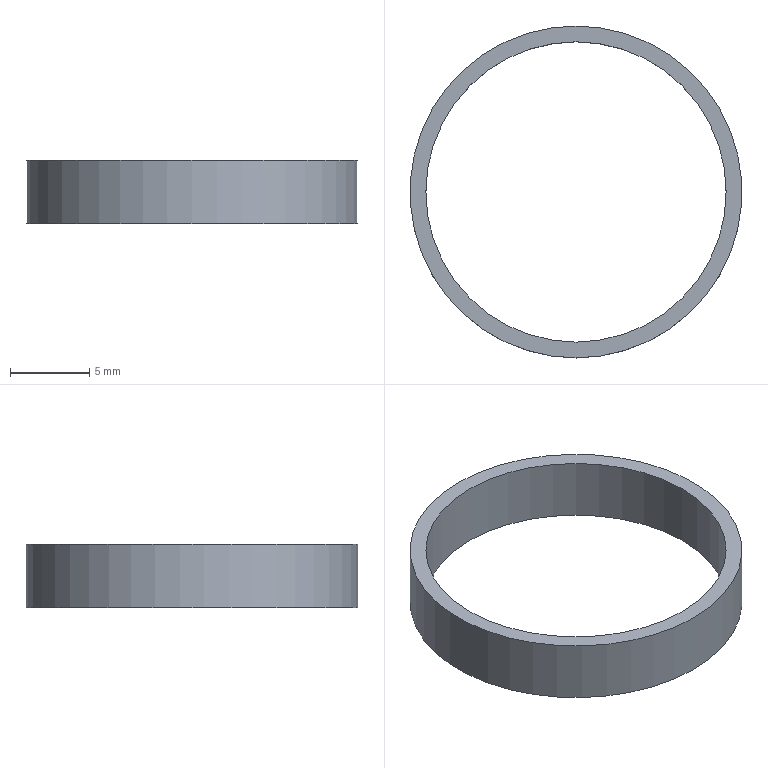Part | NX | features solid 2 | 1 solid | 4 faces | box 21 x 21 x 4 mm | volume 251.327 mm3 | cylinder 2 | plane 2 | commonest cylinder face diameters 19 x1 21 x1
STEP:
#1=CARTESIAN_POINT('',(254.748,69.5,-15.));
#2=VERTEX_POINT('',#1);
#3=CARTESIAN_POINT('',(254.748,60.,-15.));
#4=DIRECTION('',(0.,0.,-1.));
#5=DIRECTION('',(0.,1.,0.));
#6=AXIS2_PLACEMENT_3D('',#3,#4,#5);
#7=CIRCLE('',#6,9.5);
#8=EDGE_CURVE('',#2,#2,#7,.T.);
#9=ORIENTED_EDGE('',*,*,#8,.T.);
#10=EDGE_LOOP('',(#9));
#11=FACE_BOUND('',#10,.T.);
#12=CARTESIAN_POINT('',(254.748,69.5,-11.));
#13=VERTEX_POINT('',#12);
#14=CARTESIAN_POINT('',(254.748,60.,-11.));
#15=DIRECTION('',(0.,0.,-1.));
#16=DIRECTION('',(0.,1.,0.));
#17=AXIS2_PLACEMENT_3D('',#14,#15,#16);
#18=CIRCLE('',#17,9.5);
#19=EDGE_CURVE('',#13,#13,#18,.T.);
#20=ORIENTED_EDGE('',*,*,#19,.F.);
#21=EDGE_LOOP('',(#20));
#22=FACE_BOUND('',#21,.T.);
#23=CARTESIAN_POINT('',(254.748,60.,-15.));
#24=DIRECTION('',(0.,0.,1.));
#25=DIRECTION('',(0.,1.,0.));
#26=AXIS2_PLACEMENT_3D('',#23,#24,#25);
#27=CYLINDRICAL_SURFACE('',#26,9.5);
#28=ADVANCED_FACE('',(#11,#22),#27,.F.);
#29=CARTESIAN_POINT('',(254.748,70.5,-15.));
#30=VERTEX_POINT('',#29);
#31=CARTESIAN_POINT('',(254.748,60.,-15.));
#32=DIRECTION('',(0.,0.,-1.));
#33=DIRECTION('',(0.,1.,0.));
#34=AXIS2_PLACEMENT_3D('',#31,#32,#33);
#35=CIRCLE('',#34,10.5);
#36=EDGE_CURVE('',#30,#30,#35,.T.);
#37=ORIENTED_EDGE('',*,*,#36,.F.);
#38=EDGE_LOOP('',(#37));
#39=FACE_BOUND('',#38,.T.);
#40=CARTESIAN_POINT('',(254.748,70.5,-11.));
#41=VERTEX_POINT('',#40);
#42=CARTESIAN_POINT('',(254.748,60.,-11.));
#43=DIRECTION('',(0.,0.,-1.));
#44=DIRECTION('',(0.,1.,0.));
#45=AXIS2_PLACEMENT_3D('',#42,#43,#44);
#46=CIRCLE('',#45,10.5);
#47=EDGE_CURVE('',#41,#41,#46,.T.);
#48=ORIENTED_EDGE('',*,*,#47,.T.);
#49=EDGE_LOOP('',(#48));
#50=FACE_BOUND('',#49,.T.);
#51=CARTESIAN_POINT('',(254.748,60.,-15.));
#52=DIRECTION('',(0.,0.,1.));
#53=DIRECTION('',(0.,1.,0.));
#54=AXIS2_PLACEMENT_3D('',#51,#52,#53);
#55=CYLINDRICAL_SURFACE('',#54,10.5);
#56=ADVANCED_FACE('',(#39,#50),#55,.T.);
#57=ORIENTED_EDGE('',*,*,#8,.F.);
#58=EDGE_LOOP('',(#57));
#59=FACE_BOUND('',#58,.T.);
#60=ORIENTED_EDGE('',*,*,#36,.T.);
#61=EDGE_LOOP('',(#60));
#62=FACE_BOUND('',#61,.T.);
#63=CARTESIAN_POINT('',(254.748,60.,-15.));
#64=DIRECTION('',(0.,0.,-1.));
#65=DIRECTION('',(0.,-1.,0.));
#66=AXIS2_PLACEMENT_3D('',#63,#64,#65);
#67=PLANE('',#66);
#68=ADVANCED_FACE('',(#59,#62),#67,.T.);
#69=ORIENTED_EDGE('',*,*,#19,.T.);
#70=EDGE_LOOP('',(#69));
#71=FACE_BOUND('',#70,.T.);
#72=ORIENTED_EDGE('',*,*,#47,.F.);
#73=EDGE_LOOP('',(#72));
#74=FACE_BOUND('',#73,.T.);
#75=CARTESIAN_POINT('',(254.748,60.,-11.));
#76=DIRECTION('',(0.,0.,-1.));
#77=DIRECTION('',(0.,-1.,0.));
#78=AXIS2_PLACEMENT_3D('',#75,#76,#77);
#79=PLANE('',#78);
#80=ADVANCED_FACE('',(#71,#74),#79,.F.);
#81=CLOSED_SHELL('',(#28,#56,#68,#80));
#82=MANIFOLD_SOLID_BREP('',#81);
#83=(LENGTH_UNIT()NAMED_UNIT(*)SI_UNIT(.MILLI.,.METRE.));
#84=UNCERTAINTY_MEASURE_WITH_UNIT(LENGTH_MEASURE(0.00001),#83,'','');
#85=(NAMED_UNIT(*)PLANE_ANGLE_UNIT()SI_UNIT($,.RADIAN.));
#86=(NAMED_UNIT(*)SI_UNIT($,.STERADIAN.)SOLID_ANGLE_UNIT());
#87=(GEOMETRIC_REPRESENTATION_CONTEXT(3)GLOBAL_UNCERTAINTY_ASSIGNED_CONTEXT((#84))GLOBAL_UNIT_ASSIGNED_CONTEXT((#83,#85,#86))REPRESENTATION_CONTEXT('',''));
#88=ADVANCED_BREP_SHAPE_REPRESENTATION('',(#82),#87);